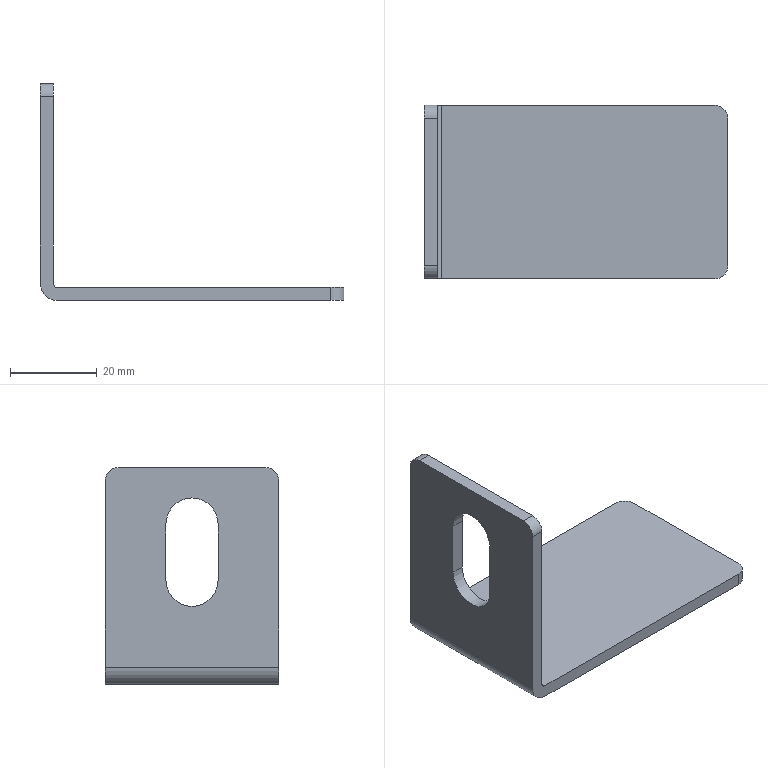Part | STEP file | E3-护栏FixedPlate 2-1 | 1 solid | 19 faces | box 70 x 40 x 50 mm | volume 13081 mm3 | plane 10 | cylinder 9 | commonest cylinder face diameters 6 x4 12 x3 2 x1 8 x1